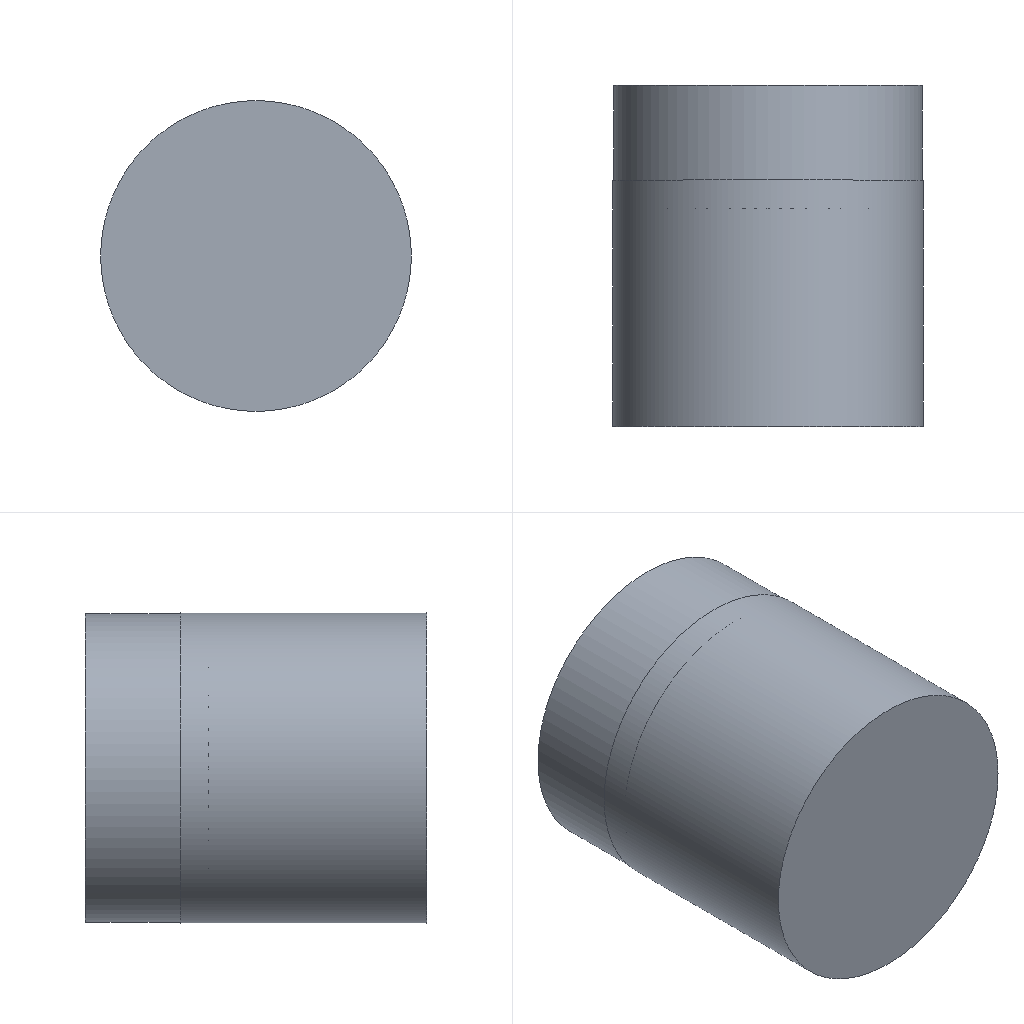Simulation study | abaqus
Set-up summary:
category,name,step,type,value,unit,region
solver,abaqus
solver,version,,,Abaqus/Explicit 2020
units,not stated in the deck,,not stated
analysis,deck,,dynamic temperature-displacement,dynamic temperature-displacement
load_step,Step-1,Step-1,dynamic temperature-displacement,nlgeom=True
contact,interactions,,,general=1 pairs=0 ties=0
load_step,requested,,,1
mesh,nodes,,,41433
mesh,elements,,,94034
element_type,S3,,shell,56
element_type,S4R,,shell,8731
element_type,C3D4T,,solid,78127
element_type,C3D8RT,,solid,7120
load,load commands in deck,,count,1
bc,support commands in deck,,count,7
material,MATERIAL-1,,in results
material,MATERIAL-2,,in results
check,setup vs results,,match,"per instance, exact: element labels, types and connectivity; labels of the nodes the elements use; coordinates of those nodes at SINGLE_PRECISION in 3 of 3 instance(s)"
Abaqus input file, long lists of numbers shortened:
*Heading
** Job name: Job-2 Model name: Model-2
** Generated by: Abaqus/CAE 2020
*Preprint, echo=NO, model=NO, history=NO, contact=NO
**
** PARTS
**
*Part, name=Parricles
*Node
      1,   11.549,   12.108,   11.876
      2,   9.671,   12.391,   11.698
** (24308 more lines like these left out)
*Element, type=C3D4T
  1, 17293, 17294,  2363, 17295
  2,  2365, 17294,  2363, 17293
** (78125 more lines like these left out)
*Nset, nset=Set-4, generate
     1,  24310,      1
*Elset, elset=Set-4, generate
     1,  78127,      1
** Section: Section-1
*Solid Section, elset=Set-4, material=Material-1
,
*End Part
**
*Part, name=chongtou
*Node
      1,  -2.918,   -12.155,          10.
      2,  -5.675,  -11.138,          10.
** (8281 more lines like these left out)
*Element, type=C3D8RT
   1,  919,  879,  948, 1013,  166,  126,  195,  260
   2,  841,  910,  784,  783,   88,  157,   31,   30
** (7118 more lines like these left out)
*Node
   8284,           0., 7.65404223e-16,           0.
*Nset, nset=chongtou-RefPt_, internal
8284,
*Nset, nset=Set-2, generate
    1,  8283,     1
*Elset, elset=Set-2, generate
    1,  7120,     1
** Section: Section-3
*Solid Section, elset=Set-2, material=Material-2
,
*End Part
**
*Part, name=rongqi
*Node
      1,   12.6,         -55.,           0.
      2,   12.6,         -35.,           0.
** (8837 more lines like these left out)
*Element, type=S4R
   1,    1,  160,  381,  161
   2,  160,  159,  382,  381
** (8729 more lines like these left out)
*Element, type=S3
6321, 8234, 8237, 6525
6322, 7901, 7802, 7614
** (54 more lines like these left out)
*Nset, nset=Set-2, generate
    1,  8839,     1
*Elset, elset=Set-2, generate
    1,  8787,     1
** Section: qiao
*Shell Section, elset=Set-2, material=Material-2
0.1, 5
*End Part
**
**
** ASSEMBLY
**
*Assembly, name=Assembly
**
*Instance, name=chongtou-1, part=chongtou
          0.,        -27.3,           0.
          0.,        -27.3,           0., 1.,        -27.3,           0., 90.
*End Instance
**
*Instance, name=rongqi-1, part=rongqi
*End Instance
**
*Instance, name=Parricles-1, part=Parricles
         -8.,         -55.,        -8.84
*End Instance
**
*Node
      1,           0.,         -55.,           0.
*Nset, nset=Set-3
 1,
*Nset, nset=Set-4, instance=chongtou-1
 8284,
*Nset, nset=b_Set-1, instance=rongqi-1, generate
    1,  8839,     1
*Elset, elset=b_Set-1, instance=rongqi-1, generate
    1,  8787,     1
*Nset, nset=b_Set-5, instance=chongtou-1, generate
    1,  8283,     1
*Elset, elset=b_Set-5, instance=chongtou-1, generate
    1,  7120,     1
*Nset, nset=_PickedSet354, internal
 1,
*Nset, nset=_PickedSet358, internal, instance=chongtou-1
 8284,
** Constraint: Constraint-1
*Rigid Body, ref node=_PickedSet354, elset=b_Set-1
** Constraint: Constraint-2
*Rigid Body, ref node=_PickedSet358, elset=b_Set-5
*End Assembly
*Amplitude, name=Amp-1
             0.,              0.,             0.1,              1.
**
** MATERIALS
**
*Material, name=Material-1
*Conductivity
10.,
*Density
 1e-09,
*Elastic
50., 0.35
*Expansion
 5e-07,
*Specific Heat
 7.8e+08,
*Material, name=Material-2
*Conductivity
46.,
*Density
 7.8e-09,
*Elastic
210000., 0.3
*Specific Heat
 4.6e+08,
**
** INTERACTION PROPERTIES
**
*Surface Interaction, name=IntProp-1
*Friction
 0.2,
*Surface Behavior, pressure-overclosure=HARD
*Gap Conductance
10000.,   0.
    0., 0.05
** ----------------------------------------------------------------
**
** STEP: Step-1
**
*Step, name=Step-1, nlgeom=YES
*Dynamic Temperature-displacement, Explicit
, 0.1
*Bulk Viscosity
0.06, 1.2
** Mass Scaling: Semi-Automatic
**               Whole Model
*Fixed Mass Scaling, factor=5000.
**
** BOUNDARY CONDITIONS
**
** Name: BC-1 Type: 对称/反对称/完全固定
*Boundary
Set-3, ENCASTRE
** Name: BC-2 Type: 位移/转角
*Boundary, amplitude=Amp-1
Set-4, 1, 1
Set-4, 2, 2, -15.
Set-4, 3, 3
Set-4, 4, 4
Set-4, 5, 5
Set-4, 6, 6
**
** INTERACTIONS
**
** Interaction: Int-1
*Contact, op=NEW
*Contact Inclusions, ALL EXTERIOR
*Contact Property Assignment
 ,  , IntProp-1
**
** OUTPUT REQUESTS
**
*Restart, write, number interval=1, time marks=NO
**
** FIELD OUTPUT: F-Output-1
**
*Output, field, number interval=50
*Node Output
A, NT, RF, RFL, U, V
*Element Output, directions=YES
EVF, HFL, LE, MISES, MISESMAX, MISESONLY, PE, PEEQ, PEEQVAVG, PEVAVG, PRESSONLY, S, SEQUT, SSAVG, SVAVG, TEMP
YIELDPOT
*Contact Output
CSTRESS,
**
** HISTORY OUTPUT: H-Output-1
**
*Output, history, variable=PRESELECT
*End Step
Results summary:
result,step,Step-1,completed,increments=32605 time=0.1/0.1
result,analysis,,,"dynamic temperature-displacement, explict"
result,last_loadstep,,,1
result,analysis steps,,count,1
result,primary field,,,"U, UR, NT11"
result,reaction total,,FX,2.31,model units
result,reaction total,,FY,18.308,model units
result,reaction total,,FZ,-10.414,model units